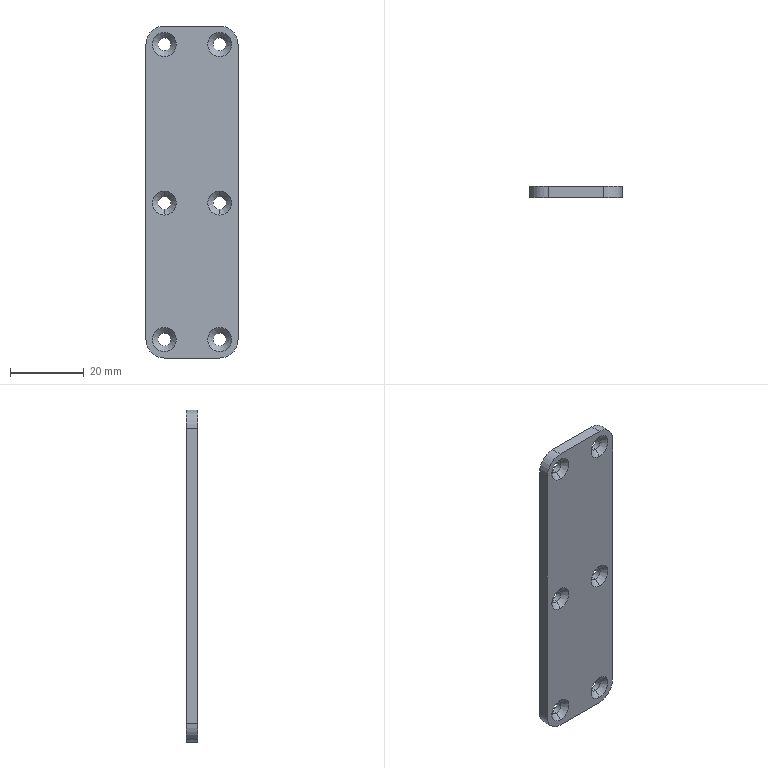Part | STEP file | 0246_208_Plate | 1 solid | 34 faces | box 25 x 3 x 90 mm | volume 6417 mm3 | cylinder 16 | cone 12 | plane 6 | commonest cylinder face diameters 3.5 x12 10 x4